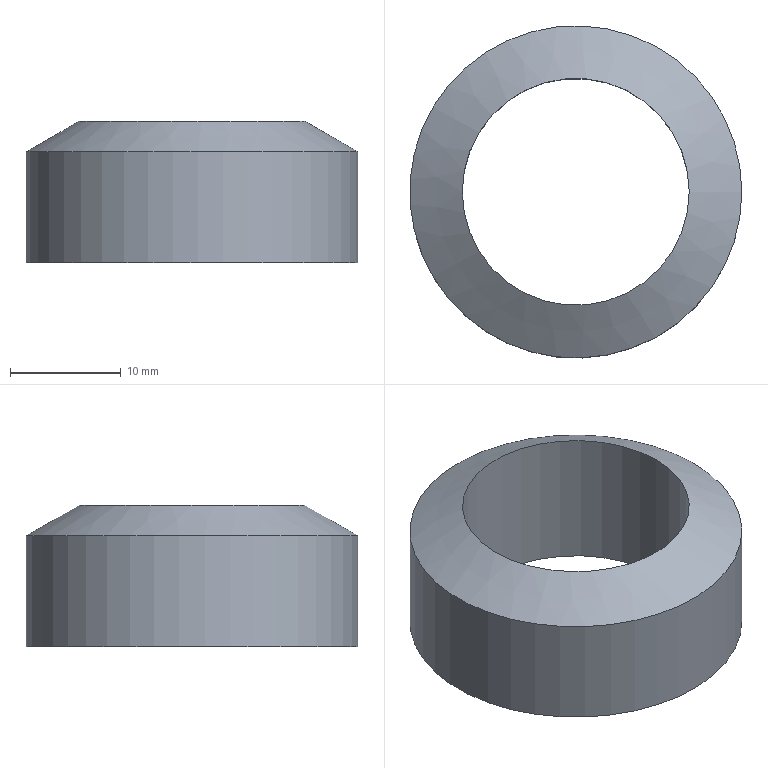Part | NX | features CYLINDER 2, CHAMFER 1, DATUM_CSYS 1 | 1 solid | 4 faces | box 30 x 30 x 12.74 mm | volume 4252 mm3 | cylinder 2 | plane 1 | cone 1 | commonest cylinder face diameters 20.5 x1 30 x1
STEP:
#1=CARTESIAN_POINT('',(10.25,0.,0.));
#2=VERTEX_POINT('',#1);
#3=CARTESIAN_POINT('',(0.,0.,0.));
#4=DIRECTION('',(0.,0.,1.));
#5=DIRECTION('',(1.,0.,0.));
#6=AXIS2_PLACEMENT_3D('',#3,#4,#5);
#7=CIRCLE('',#6,10.25);
#8=EDGE_CURVE('',#2,#2,#7,.T.);
#9=ORIENTED_EDGE('',*,*,#8,.T.);
#10=EDGE_LOOP('',(#9));
#11=FACE_BOUND('',#10,.T.);
#12=CARTESIAN_POINT('',(15.,0.,0.));
#13=VERTEX_POINT('',#12);
#14=CARTESIAN_POINT('',(0.,0.,0.));
#15=DIRECTION('',(0.,0.,1.));
#16=DIRECTION('',(1.,0.,0.));
#17=AXIS2_PLACEMENT_3D('',#14,#15,#16);
#18=CIRCLE('',#17,15.);
#19=EDGE_CURVE('',#13,#13,#18,.T.);
#20=ORIENTED_EDGE('',*,*,#19,.F.);
#21=EDGE_LOOP('',(#20));
#22=FACE_BOUND('',#21,.T.);
#23=CARTESIAN_POINT('',(0.,0.,0.));
#24=DIRECTION('',(0.,0.,-1.));
#25=DIRECTION('',(-1.,0.,0.));
#26=AXIS2_PLACEMENT_3D('',#23,#24,#25);
#27=PLANE('',#26);
#28=ADVANCED_FACE('',(#11,#22),#27,.T.);
#29=CARTESIAN_POINT('',(15.,0.,10.));
#30=VERTEX_POINT('',#29);
#31=CARTESIAN_POINT('',(0.,0.,10.));
#32=DIRECTION('',(0.,0.,1.));
#33=DIRECTION('',(1.,0.,0.));
#34=AXIS2_PLACEMENT_3D('',#31,#32,#33);
#35=CIRCLE('',#34,15.);
#36=EDGE_CURVE('',#30,#30,#35,.F.);
#37=ORIENTED_EDGE('',*,*,#36,.T.);
#38=EDGE_LOOP('',(#37));
#39=FACE_BOUND('',#38,.T.);
#40=ORIENTED_EDGE('',*,*,#19,.T.);
#41=EDGE_LOOP('',(#40));
#42=FACE_BOUND('',#41,.T.);
#43=CARTESIAN_POINT('',(0.,0.,0.));
#44=DIRECTION('',(0.,0.,1.));
#45=DIRECTION('',(1.,0.,0.));
#46=AXIS2_PLACEMENT_3D('',#43,#44,#45);
#47=CYLINDRICAL_SURFACE('',#46,15.);
#48=ADVANCED_FACE('',(#39,#42),#47,.T.);
#49=CARTESIAN_POINT('',(10.25,0.,12.74));
#50=VERTEX_POINT('',#49);
#51=CARTESIAN_POINT('',(0.,0.,12.74));
#52=DIRECTION('',(0.,0.,-1.));
#53=DIRECTION('',(1.,0.,0.));
#54=AXIS2_PLACEMENT_3D('',#51,#52,#53);
#55=CIRCLE('',#54,10.25);
#56=EDGE_CURVE('',#50,#50,#55,.T.);
#57=ORIENTED_EDGE('',*,*,#56,.F.);
#58=EDGE_LOOP('',(#57));
#59=FACE_BOUND('',#58,.T.);
#60=ORIENTED_EDGE('',*,*,#8,.F.);
#61=EDGE_LOOP('',(#60));
#62=FACE_BOUND('',#61,.T.);
#63=CARTESIAN_POINT('',(0.,0.,0.));
#64=DIRECTION('',(0.,0.,1.));
#65=DIRECTION('',(1.,0.,0.));
#66=AXIS2_PLACEMENT_3D('',#63,#64,#65);
#67=CYLINDRICAL_SURFACE('',#66,10.25);
#68=ADVANCED_FACE('',(#59,#62),#67,.F.);
#69=ORIENTED_EDGE('',*,*,#56,.T.);
#70=EDGE_LOOP('',(#69));
#71=FACE_BOUND('',#70,.T.);
#72=ORIENTED_EDGE('',*,*,#36,.F.);
#73=EDGE_LOOP('',(#72));
#74=FACE_BOUND('',#73,.T.);
#75=CARTESIAN_POINT('',(0.,0.,10.));
#76=DIRECTION('',(0.,0.,-1.));
#77=DIRECTION('',(-1.,0.,0.));
#78=AXIS2_PLACEMENT_3D('',#75,#76,#77);
#79=CONICAL_SURFACE('',#78,15.,1.048);
#80=ADVANCED_FACE('',(#71,#74),#79,.T.);
#81=CLOSED_SHELL('',(#28,#48,#68,#80));
#82=MANIFOLD_SOLID_BREP('',#81);
#83=(LENGTH_UNIT()NAMED_UNIT(*)SI_UNIT(.MILLI.,.METRE.));
#84=UNCERTAINTY_MEASURE_WITH_UNIT(LENGTH_MEASURE(0.00001),#83,'','');
#85=(NAMED_UNIT(*)PLANE_ANGLE_UNIT()SI_UNIT($,.RADIAN.));
#86=(NAMED_UNIT(*)SI_UNIT($,.STERADIAN.)SOLID_ANGLE_UNIT());
#87=(GEOMETRIC_REPRESENTATION_CONTEXT(3)GLOBAL_UNCERTAINTY_ASSIGNED_CONTEXT((#84))GLOBAL_UNIT_ASSIGNED_CONTEXT((#83,#85,#86))REPRESENTATION_CONTEXT('',''));
#88=ADVANCED_BREP_SHAPE_REPRESENTATION('',(#82),#87);